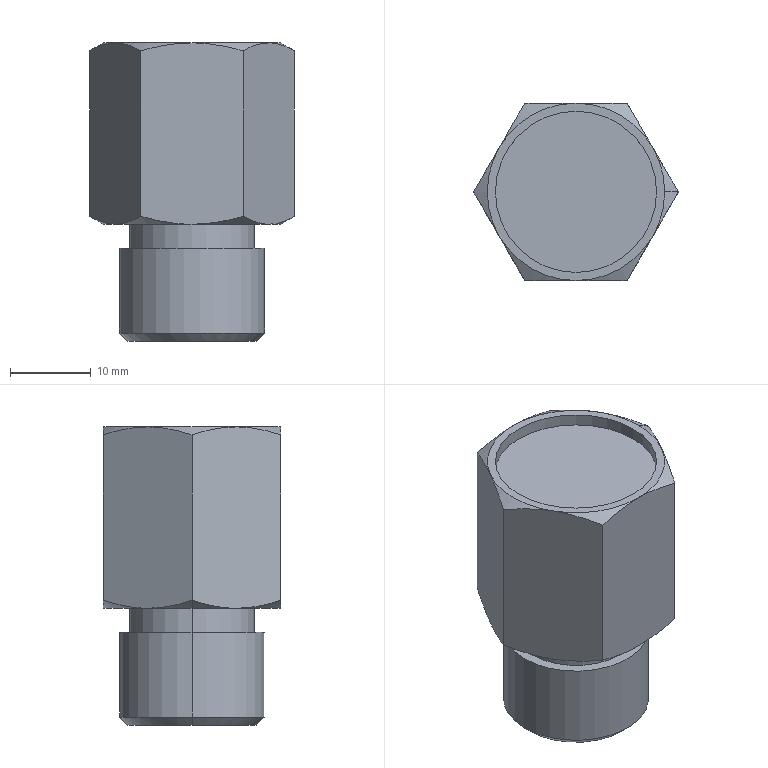Part | SolidWorks | features BaseBody 1 | 1 solid | 36 faces | box 25.403 x 22 x 37 mm | volume 8726 mm3 | cone 16 | plane 12 | cylinder 8 | commonest cylinder face diameters 12 x2 15.5 x2 18 x2 20 x2
STEP:
#1=CARTESIAN_POINT('',(180.5,0.,57.15));
#2=VERTEX_POINT('',#1);
#3=CARTESIAN_POINT('',(164.5,0.,57.15));
#4=VERTEX_POINT('',#3);
#5=CARTESIAN_POINT('',(172.5,0.,57.15));
#6=DIRECTION('',(0.,0.,-1.));
#7=DIRECTION('',(-1.,0.,0.));
#8=AXIS2_PLACEMENT_3D('',#5,#6,#7);
#9=CIRCLE('',#8,8.);
#10=EDGE_CURVE('',#2,#4,#9,.T.);
#11=ORIENTED_EDGE('',*,*,#10,.F.);
#12=CARTESIAN_POINT('',(181.5,0.,58.15));
#13=VERTEX_POINT('',#12);
#14=CARTESIAN_POINT('',(180.5,0.,57.15));
#15=DIRECTION('',(0.7071,0.,0.7071));
#16=VECTOR('',#15,1000.);
#17=LINE('',#14,#16);
#18=EDGE_CURVE('',#2,#13,#17,.T.);
#19=ORIENTED_EDGE('',*,*,#18,.T.);
#20=CARTESIAN_POINT('',(163.5,0.,58.15));
#21=VERTEX_POINT('',#20);
#22=CARTESIAN_POINT('',(172.5,0.,58.15));
#23=DIRECTION('',(0.,0.,1.));
#24=DIRECTION('',(-1.,0.,0.));
#25=AXIS2_PLACEMENT_3D('',#22,#23,#24);
#26=CIRCLE('',#25,9.);
#27=EDGE_CURVE('',#21,#13,#26,.T.);
#28=ORIENTED_EDGE('',*,*,#27,.F.);
#29=CARTESIAN_POINT('',(164.5,0.,57.15));
#30=DIRECTION('',(-0.7071,0.,0.7071));
#31=VECTOR('',#30,1000.);
#32=LINE('',#29,#31);
#33=EDGE_CURVE('',#4,#21,#32,.T.);
#34=ORIENTED_EDGE('',*,*,#33,.F.);
#35=EDGE_LOOP('',(#11,#19,#28,#34));
#36=FACE_OUTER_BOUND('',#35,.T.);
#37=CARTESIAN_POINT('',(172.5,0.,57.15));
#38=DIRECTION('',(0.,0.,1.));
#39=DIRECTION('',(-1.,0.,0.));
#40=AXIS2_PLACEMENT_3D('',#37,#38,#39);
#41=CONICAL_SURFACE('',#40,8.,0.7854);
#42=ADVANCED_FACE('',(#36),#41,.T.);
#43=CARTESIAN_POINT('',(166.5,0.,89.65));
#44=VERTEX_POINT('',#43);
#45=CARTESIAN_POINT('',(178.5,0.,89.65));
#46=VERTEX_POINT('',#45);
#47=CARTESIAN_POINT('',(172.5,0.,89.65));
#48=DIRECTION('',(0.,0.,-1.));
#49=DIRECTION('',(1.,0.,0.));
#50=AXIS2_PLACEMENT_3D('',#47,#48,#49);
#51=CIRCLE('',#50,6.);
#52=EDGE_CURVE('',#44,#46,#51,.T.);
#53=ORIENTED_EDGE('',*,*,#52,.F.);
#54=CARTESIAN_POINT('',(166.5,0.,57.15));
#55=VERTEX_POINT('',#54);
#56=CARTESIAN_POINT('',(166.5,0.,89.65));
#57=DIRECTION('',(0.,0.,-1.));
#58=VECTOR('',#57,1000.);
#59=LINE('',#56,#58);
#60=EDGE_CURVE('',#44,#55,#59,.T.);
#61=ORIENTED_EDGE('',*,*,#60,.T.);
#62=CARTESIAN_POINT('',(178.5,0.,57.15));
#63=VERTEX_POINT('',#62);
#64=CARTESIAN_POINT('',(172.5,0.,57.15));
#65=DIRECTION('',(0.,0.,-1.));
#66=DIRECTION('',(1.,0.,0.));
#67=AXIS2_PLACEMENT_3D('',#64,#65,#66);
#68=CIRCLE('',#67,6.);
#69=EDGE_CURVE('',#55,#63,#68,.T.);
#70=ORIENTED_EDGE('',*,*,#69,.T.);
#71=CARTESIAN_POINT('',(178.5,0.,89.65));
#72=DIRECTION('',(0.,0.,-1.));
#73=VECTOR('',#72,1000.);
#74=LINE('',#71,#73);
#75=EDGE_CURVE('',#46,#63,#74,.T.);
#76=ORIENTED_EDGE('',*,*,#75,.F.);
#77=EDGE_LOOP('',(#53,#61,#70,#76));
#78=FACE_OUTER_BOUND('',#77,.T.);
#79=CARTESIAN_POINT('',(172.5,0.,89.65));
#80=DIRECTION('',(0.,0.,-1.));
#81=DIRECTION('',(1.,0.,0.));
#82=AXIS2_PLACEMENT_3D('',#79,#80,#81);
#83=CYLINDRICAL_SURFACE('',#82,6.);
#84=ADVANCED_FACE('',(#78),#83,.F.);
#85=CARTESIAN_POINT('',(163.5,0.,68.65));
#86=VERTEX_POINT('',#85);
#87=CARTESIAN_POINT('',(181.5,0.,68.65));
#88=VERTEX_POINT('',#87);
#89=CARTESIAN_POINT('',(172.5,0.,68.65));
#90=DIRECTION('',(0.,0.,1.));
#91=DIRECTION('',(-1.,0.,0.));
#92=AXIS2_PLACEMENT_3D('',#89,#90,#91);
#93=CIRCLE('',#92,9.);
#94=EDGE_CURVE('',#86,#88,#93,.T.);
#95=ORIENTED_EDGE('',*,*,#94,.F.);
#96=CARTESIAN_POINT('',(163.5,0.,71.65));
#97=DIRECTION('',(0.,0.,-1.));
#98=VECTOR('',#97,1000.);
#99=LINE('',#96,#98);
#100=EDGE_CURVE('',#86,#21,#99,.T.);
#101=ORIENTED_EDGE('',*,*,#100,.T.);
#102=ORIENTED_EDGE('',*,*,#27,.T.);
#103=CARTESIAN_POINT('',(181.5,0.,71.65));
#104=DIRECTION('',(0.,0.,-1.));
#105=VECTOR('',#104,1000.);
#106=LINE('',#103,#105);
#107=EDGE_CURVE('',#88,#13,#106,.T.);
#108=ORIENTED_EDGE('',*,*,#107,.F.);
#109=EDGE_LOOP('',(#95,#101,#102,#108));
#110=FACE_OUTER_BOUND('',#109,.T.);
#111=CARTESIAN_POINT('',(172.5,0.,71.65));
#112=DIRECTION('',(0.,0.,-1.));
#113=DIRECTION('',(1.,0.,0.));
#114=AXIS2_PLACEMENT_3D('',#111,#112,#113);
#115=CYLINDRICAL_SURFACE('',#114,9.);
#116=ADVANCED_FACE('',(#110),#115,.T.);
#117=CARTESIAN_POINT('',(164.75,0.,68.65));
#118=VERTEX_POINT('',#117);
#119=CARTESIAN_POINT('',(180.25,0.,68.65));
#120=VERTEX_POINT('',#119);
#121=CARTESIAN_POINT('',(172.5,0.,68.65));
#122=DIRECTION('',(0.,0.,1.));
#123=DIRECTION('',(-1.,0.,0.));
#124=AXIS2_PLACEMENT_3D('',#121,#122,#123);
#125=CIRCLE('',#124,7.75);
#126=EDGE_CURVE('',#118,#120,#125,.T.);
#127=ORIENTED_EDGE('',*,*,#126,.T.);
#128=CARTESIAN_POINT('',(180.25,0.,71.65));
#129=VERTEX_POINT('',#128);
#130=CARTESIAN_POINT('',(180.25,0.,94.15));
#131=DIRECTION('',(0.,0.,1.));
#132=VECTOR('',#131,1000.);
#133=LINE('',#130,#132);
#134=EDGE_CURVE('',#120,#129,#133,.T.);
#135=ORIENTED_EDGE('',*,*,#134,.T.);
#136=CARTESIAN_POINT('',(164.75,0.,71.65));
#137=VERTEX_POINT('',#136);
#138=CARTESIAN_POINT('',(172.5,0.,71.65));
#139=DIRECTION('',(0.,0.,1.));
#140=DIRECTION('',(-1.,0.,0.));
#141=AXIS2_PLACEMENT_3D('',#138,#139,#140);
#142=CIRCLE('',#141,7.75);
#143=EDGE_CURVE('',#137,#129,#142,.T.);
#144=ORIENTED_EDGE('',*,*,#143,.F.);
#145=CARTESIAN_POINT('',(164.75,0.,94.15));
#146=DIRECTION('',(0.,0.,1.));
#147=VECTOR('',#146,1000.);
#148=LINE('',#145,#147);
#149=EDGE_CURVE('',#118,#137,#148,.T.);
#150=ORIENTED_EDGE('',*,*,#149,.F.);
#151=EDGE_LOOP('',(#127,#135,#144,#150));
#152=FACE_OUTER_BOUND('',#151,.T.);
#153=CARTESIAN_POINT('',(172.5,0.,94.15));
#154=DIRECTION('',(0.,0.,1.));
#155=DIRECTION('',(-1.,0.,0.));
#156=AXIS2_PLACEMENT_3D('',#153,#154,#155);
#157=CYLINDRICAL_SURFACE('',#156,7.75);
#158=ADVANCED_FACE('',(#152),#157,.T.);
#159=CARTESIAN_POINT('',(182.5,0.,92.65));
#160=VERTEX_POINT('',#159);
#161=CARTESIAN_POINT('',(162.5,0.,92.65));
#162=VERTEX_POINT('',#161);
#163=CARTESIAN_POINT('',(172.5,0.,92.65));
#164=DIRECTION('',(0.,0.,1.));
#165=DIRECTION('',(-1.,0.,0.));
#166=AXIS2_PLACEMENT_3D('',#163,#164,#165);
#167=CIRCLE('',#166,10.);
#168=EDGE_CURVE('',#160,#162,#167,.T.);
#169=ORIENTED_EDGE('',*,*,#168,.F.);
#170=CARTESIAN_POINT('',(182.5,0.,94.15));
#171=VERTEX_POINT('',#170);
#172=CARTESIAN_POINT('',(182.5,0.,92.65));
#173=DIRECTION('',(0.,0.,1.));
#174=VECTOR('',#173,1000.);
#175=LINE('',#172,#174);
#176=EDGE_CURVE('',#160,#171,#175,.T.);
#177=ORIENTED_EDGE('',*,*,#176,.T.);
#178=CARTESIAN_POINT('',(162.5,0.,94.15));
#179=VERTEX_POINT('',#178);
#180=CARTESIAN_POINT('',(172.5,0.,94.15));
#181=DIRECTION('',(0.,0.,1.));
#182=DIRECTION('',(-1.,0.,0.));
#183=AXIS2_PLACEMENT_3D('',#180,#181,#182);
#184=CIRCLE('',#183,10.);
#185=EDGE_CURVE('',#171,#179,#184,.T.);
#186=ORIENTED_EDGE('',*,*,#185,.T.);
#187=CARTESIAN_POINT('',(162.5,0.,92.65));
#188=DIRECTION('',(0.,0.,1.));
#189=VECTOR('',#188,1000.);
#190=LINE('',#187,#189);
#191=EDGE_CURVE('',#162,#179,#190,.T.);
#192=ORIENTED_EDGE('',*,*,#191,.F.);
#193=EDGE_LOOP('',(#169,#177,#186,#192));
#194=FACE_OUTER_BOUND('',#193,.T.);
#195=CARTESIAN_POINT('',(172.5,0.,92.65));
#196=DIRECTION('',(0.,0.,1.));
#197=DIRECTION('',(-1.,0.,0.));
#198=AXIS2_PLACEMENT_3D('',#195,#196,#197);
#199=CYLINDRICAL_SURFACE('',#198,10.);
#200=ADVANCED_FACE('',(#194),#199,.F.);
#201=CARTESIAN_POINT('',(183.5,0.,94.15));
#202=VERTEX_POINT('',#201);
#203=CARTESIAN_POINT('',(182.026,5.5,94.15));
#204=VERTEX_POINT('',#203);
#205=CARTESIAN_POINT('',(172.5,0.,94.15));
#206=DIRECTION('',(0.,0.,1.));
#207=DIRECTION('',(-1.,0.,0.));
#208=AXIS2_PLACEMENT_3D('',#205,#206,#207);
#209=CIRCLE('',#208,11.);
#210=EDGE_CURVE('',#202,#204,#209,.T.);
#211=ORIENTED_EDGE('',*,*,#210,.F.);
#212=CARTESIAN_POINT('',(185.202,0.,93.168));
#213=VERTEX_POINT('',#212);
#214=CARTESIAN_POINT('',(183.5,0.,94.15));
#215=DIRECTION('',(0.866,0.,-0.5));
#216=VECTOR('',#215,1000.);
#217=LINE('',#214,#216);
#218=EDGE_CURVE('',#202,#213,#217,.T.);
#219=ORIENTED_EDGE('',*,*,#218,.T.);
#220=CARTESIAN_POINT('',(185.202,0.,93.168));
#221=CARTESIAN_POINT('',(184.682,0.8997,93.467));
#222=CARTESIAN_POINT('',(184.159,1.806,93.715));
#223=CARTESIAN_POINT('',(183.102,3.638,94.056));
#224=CARTESIAN_POINT('',(182.567,4.563,94.15));
#225=CARTESIAN_POINT('',(182.026,5.5,94.15));
#226=B_SPLINE_CURVE_WITH_KNOTS('',3,(#220,#221,#222,#223,#224,#225),.UNSPECIFIED.,.F.,.F.,(4,2,4),(0.000000238,0.003213,0.006426),.UNSPECIFIED.);
#227=EDGE_CURVE('',#213,#204,#226,.T.);
#228=ORIENTED_EDGE('',*,*,#227,.T.);
#229=EDGE_LOOP('',(#211,#219,#228));
#230=FACE_OUTER_BOUND('',#229,.T.);
#231=CARTESIAN_POINT('',(172.5,0.,94.15));
#232=DIRECTION('',(0.,0.,-1.));
#233=DIRECTION('',(1.,0.,0.));
#234=AXIS2_PLACEMENT_3D('',#231,#232,#233);
#235=CONICAL_SURFACE('',#234,11.,1.047);
#236=ADVANCED_FACE('',(#230),#235,.T.);
#237=CARTESIAN_POINT('',(161.5,0.,71.65));
#238=VERTEX_POINT('',#237);
#239=CARTESIAN_POINT('',(162.974,5.5,71.65));
#240=VERTEX_POINT('',#239);
#241=CARTESIAN_POINT('',(172.5,0.,71.65));
#242=DIRECTION('',(0.,0.,-1.));
#243=DIRECTION('',(1.,0.,0.));
#244=AXIS2_PLACEMENT_3D('',#241,#242,#243);
#245=CIRCLE('',#244,11.);
#246=EDGE_CURVE('',#238,#240,#245,.T.);
#247=ORIENTED_EDGE('',*,*,#246,.F.);
#248=CARTESIAN_POINT('',(159.798,0.,72.632));
#249=VERTEX_POINT('',#248);
#250=CARTESIAN_POINT('',(159.798,0.,72.632));
#251=DIRECTION('',(-0.866,0.,0.5));
#252=VECTOR('',#251,1000.);
#253=LINE('',#250,#252);
#254=EDGE_CURVE('',#238,#249,#253,.T.);
#255=ORIENTED_EDGE('',*,*,#254,.T.);
#256=CARTESIAN_POINT('',(159.798,0.,72.632));
#257=CARTESIAN_POINT('',(160.318,0.8997,72.333));
#258=CARTESIAN_POINT('',(160.841,1.806,72.085));
#259=CARTESIAN_POINT('',(161.898,3.638,71.744));
#260=CARTESIAN_POINT('',(162.433,4.563,71.65));
#261=CARTESIAN_POINT('',(162.974,5.5,71.65));
#262=B_SPLINE_CURVE_WITH_KNOTS('',3,(#256,#257,#258,#259,#260,#261),.UNSPECIFIED.,.F.,.F.,(4,2,4),(0.000000238,0.003213,0.006426),.UNSPECIFIED.);
#263=EDGE_CURVE('',#249,#240,#262,.T.);
#264=ORIENTED_EDGE('',*,*,#263,.T.);
#265=EDGE_LOOP('',(#247,#255,#264));
#266=FACE_OUTER_BOUND('',#265,.T.);
#267=CARTESIAN_POINT('',(172.5,0.,72.632));
#268=DIRECTION('',(0.,0.,1.));
#269=DIRECTION('',(-1.,0.,0.));
#270=AXIS2_PLACEMENT_3D('',#267,#268,#269);
#271=CONICAL_SURFACE('',#270,12.702,1.047);
#272=ADVANCED_FACE('',(#266),#271,.T.);
#273=CARTESIAN_POINT('',(159.798,0.,93.168));
#274=VERTEX_POINT('',#273);
#275=CARTESIAN_POINT('',(162.974,-5.5,94.15));
#276=VERTEX_POINT('',#275);
#277=CARTESIAN_POINT('',(159.798,0.,93.168));
#278=CARTESIAN_POINT('',(160.318,-0.8997,93.467));
#279=CARTESIAN_POINT('',(160.841,-1.806,93.715));
#280=CARTESIAN_POINT('',(161.898,-3.638,94.056));
#281=CARTESIAN_POINT('',(162.433,-4.563,94.15));
#282=CARTESIAN_POINT('',(162.974,-5.5,94.15));
#283=B_SPLINE_CURVE_WITH_KNOTS('',3,(#277,#278,#279,#280,#281,#282),.UNSPECIFIED.,.F.,.F.,(4,2,4),(0.000000238,0.003213,0.006426),.UNSPECIFIED.);
#284=EDGE_CURVE('',#274,#276,#283,.T.);
#285=ORIENTED_EDGE('',*,*,#284,.F.);
#286=CARTESIAN_POINT('',(159.798,0.,57.15));
#287=DIRECTION('',(0.,0.,1.));
#288=VECTOR('',#287,1000.);
#289=LINE('',#286,#288);
#290=EDGE_CURVE('',#249,#274,#289,.T.);
#291=ORIENTED_EDGE('',*,*,#290,.F.);
#292=CARTESIAN_POINT('',(162.974,-5.5,71.65));
#293=VERTEX_POINT('',#292);
#294=CARTESIAN_POINT('',(162.974,-5.5,71.65));
#295=CARTESIAN_POINT('',(162.704,-5.033,71.65));
#296=CARTESIAN_POINT('',(162.434,-4.564,71.673));
#297=CARTESIAN_POINT('',(161.898,-3.637,71.763));
#298=CARTESIAN_POINT('',(161.632,-3.176,71.83));
#299=CARTESIAN_POINT('',(160.839,-1.802,72.086));
#300=CARTESIAN_POINT('',(160.316,-0.8975,72.333));
#301=CARTESIAN_POINT('',(159.798,0.,72.632));
#302=B_SPLINE_CURVE_WITH_KNOTS('',3,(#294,#295,#296,#297,#298,#299,#300,#301),.UNSPECIFIED.,.F.,.F.,(4,2,2,4),(0.006426,0.008027,0.009627,0.01283),.UNSPECIFIED.);
#303=EDGE_CURVE('',#293,#249,#302,.T.);
#304=ORIENTED_EDGE('',*,*,#303,.F.);
#305=CARTESIAN_POINT('',(166.149,-11.,72.632));
#306=VERTEX_POINT('',#305);
#307=CARTESIAN_POINT('',(166.149,-11.,72.632));
#308=CARTESIAN_POINT('',(165.63,-10.1,72.333));
#309=CARTESIAN_POINT('',(165.106,-9.194,72.085));
#310=CARTESIAN_POINT('',(164.049,-7.362,71.744));
#311=CARTESIAN_POINT('',(163.515,-6.437,71.65));
#312=CARTESIAN_POINT('',(162.974,-5.5,71.65));
#313=B_SPLINE_CURVE_WITH_KNOTS('',3,(#307,#308,#309,#310,#311,#312),.UNSPECIFIED.,.F.,.F.,(4,2,4),(0.000000238,0.003213,0.006426),.UNSPECIFIED.);
#314=EDGE_CURVE('',#306,#293,#313,.T.);
#315=ORIENTED_EDGE('',*,*,#314,.F.);
#316=CARTESIAN_POINT('',(166.149,-11.,93.168));
#317=VERTEX_POINT('',#316);
#318=CARTESIAN_POINT('',(166.149,-11.,57.15));
#319=DIRECTION('',(0.,0.,1.));
#320=VECTOR('',#319,1000.);
#321=LINE('',#318,#320);
#322=EDGE_CURVE('',#306,#317,#321,.T.);
#323=ORIENTED_EDGE('',*,*,#322,.T.);
#324=CARTESIAN_POINT('',(162.974,-5.5,94.15));
#325=CARTESIAN_POINT('',(163.243,-5.967,94.15));
#326=CARTESIAN_POINT('',(163.514,-6.436,94.127));
#327=CARTESIAN_POINT('',(164.049,-7.363,94.037));
#328=CARTESIAN_POINT('',(164.315,-7.824,93.97));
#329=CARTESIAN_POINT('',(165.109,-9.198,93.714));
#330=CARTESIAN_POINT('',(165.631,-10.103,93.467));
#331=CARTESIAN_POINT('',(166.149,-11.,93.168));
#332=B_SPLINE_CURVE_WITH_KNOTS('',3,(#324,#325,#326,#327,#328,#329,#330,#331),.UNSPECIFIED.,.F.,.F.,(4,2,2,4),(0.006426,0.008027,0.009627,0.01283),.UNSPECIFIED.);
#333=EDGE_CURVE('',#276,#317,#332,.T.);
#334=ORIENTED_EDGE('',*,*,#333,.F.);
#335=EDGE_LOOP('',(#285,#291,#304,#315,#323,#334));
#336=FACE_OUTER_BOUND('',#335,.T.);
#337=CARTESIAN_POINT('',(166.149,-11.,57.15));
#338=DIRECTION('',(0.866,0.5,0.));
#339=DIRECTION('',(0.5,-0.866,0.));
#340=AXIS2_PLACEMENT_3D('',#337,#338,#339);
#341=PLANE('',#340);
#342=ADVANCED_FACE('',(#336),#341,.F.);
#343=CARTESIAN_POINT('',(166.149,11.,93.168));
#344=VERTEX_POINT('',#343);
#345=CARTESIAN_POINT('',(162.974,5.5,94.15));
#346=VERTEX_POINT('',#345);
#347=CARTESIAN_POINT('',(166.149,11.,93.168));
#348=CARTESIAN_POINT('',(165.63,10.1,93.467));
#349=CARTESIAN_POINT('',(165.106,9.194,93.715));
#350=CARTESIAN_POINT('',(164.049,7.362,94.056));
#351=CARTESIAN_POINT('',(163.515,6.437,94.15));
#352=CARTESIAN_POINT('',(162.974,5.5,94.15));
#353=B_SPLINE_CURVE_WITH_KNOTS('',3,(#347,#348,#349,#350,#351,#352),.UNSPECIFIED.,.F.,.F.,(4,2,4),(0.000000238,0.003213,0.006426),.UNSPECIFIED.);
#354=EDGE_CURVE('',#344,#346,#353,.T.);
#355=ORIENTED_EDGE('',*,*,#354,.F.);
#356=CARTESIAN_POINT('',(166.149,11.,72.632));
#357=VERTEX_POINT('',#356);
#358=CARTESIAN_POINT('',(166.149,11.,57.15));
#359=DIRECTION('',(0.,0.,1.));
#360=VECTOR('',#359,1000.);
#361=LINE('',#358,#360);
#362=EDGE_CURVE('',#357,#344,#361,.T.);
#363=ORIENTED_EDGE('',*,*,#362,.F.);
#364=CARTESIAN_POINT('',(162.974,5.5,71.65));
#365=CARTESIAN_POINT('',(163.243,5.967,71.65));
#366=CARTESIAN_POINT('',(163.514,6.436,71.673));
#367=CARTESIAN_POINT('',(164.049,7.363,71.763));
#368=CARTESIAN_POINT('',(164.315,7.824,71.83));
#369=CARTESIAN_POINT('',(165.109,9.198,72.086));
#370=CARTESIAN_POINT('',(165.631,10.103,72.333));
#371=CARTESIAN_POINT('',(166.149,11.,72.632));
#372=B_SPLINE_CURVE_WITH_KNOTS('',3,(#364,#365,#366,#367,#368,#369,#370,#371),.UNSPECIFIED.,.F.,.F.,(4,2,2,4),(0.006426,0.008027,0.009627,0.01283),.UNSPECIFIED.);
#373=EDGE_CURVE('',#240,#357,#372,.T.);
#374=ORIENTED_EDGE('',*,*,#373,.F.);
#375=ORIENTED_EDGE('',*,*,#263,.F.);
#376=ORIENTED_EDGE('',*,*,#290,.T.);
#377=CARTESIAN_POINT('',(162.974,5.5,94.15));
#378=CARTESIAN_POINT('',(162.704,5.033,94.15));
#379=CARTESIAN_POINT('',(162.434,4.564,94.127));
#380=CARTESIAN_POINT('',(161.898,3.637,94.037));
#381=CARTESIAN_POINT('',(161.632,3.176,93.97));
#382=CARTESIAN_POINT('',(160.839,1.802,93.714));
#383=CARTESIAN_POINT('',(160.316,0.8975,93.467));
#384=CARTESIAN_POINT('',(159.798,0.,93.168));
#385=B_SPLINE_CURVE_WITH_KNOTS('',3,(#377,#378,#379,#380,#381,#382,#383,#384),.UNSPECIFIED.,.F.,.F.,(4,2,2,4),(0.006426,0.008027,0.009627,0.01283),.UNSPECIFIED.);
#386=EDGE_CURVE('',#346,#274,#385,.T.);
#387=ORIENTED_EDGE('',*,*,#386,.F.);
#388=EDGE_LOOP('',(#355,#363,#374,#375,#376,#387));
#389=FACE_OUTER_BOUND('',#388,.T.);
#390=CARTESIAN_POINT('',(159.798,0.,57.15));
#391=DIRECTION('',(0.866,-0.5,0.));
#392=DIRECTION('',(-0.5,-0.866,0.));
#393=AXIS2_PLACEMENT_3D('',#390,#391,#392);
#394=PLANE('',#393);
#395=ADVANCED_FACE('',(#389),#394,.F.);
#396=CARTESIAN_POINT('',(178.851,11.,93.168));
#397=VERTEX_POINT('',#396);
#398=CARTESIAN_POINT('',(172.5,11.,94.15));
#399=VERTEX_POINT('',#398);
#400=CARTESIAN_POINT('',(178.851,11.,93.168));
#401=CARTESIAN_POINT('',(177.824,11.,93.464));
#402=CARTESIAN_POINT('',(176.784,11.,93.711));
#403=CARTESIAN_POINT('',(175.193,11.,93.969));
#404=CARTESIAN_POINT('',(174.656,11.,94.037));
#405=CARTESIAN_POINT('',(173.576,11.,94.127));
#406=CARTESIAN_POINT('',(173.037,11.,94.15));
#407=CARTESIAN_POINT('',(172.5,11.,94.15));
#408=B_SPLINE_CURVE_WITH_KNOTS('',3,(#400,#401,#402,#403,#404,#405,#406,#407),.UNSPECIFIED.,.F.,.F.,(4,2,2,4),(0.004655,0.007861,0.009464,0.01107),.UNSPECIFIED.);
#409=EDGE_CURVE('',#397,#399,#408,.T.);
#410=ORIENTED_EDGE('',*,*,#409,.F.);
#411=CARTESIAN_POINT('',(178.851,11.,72.632));
#412=VERTEX_POINT('',#411);
#413=CARTESIAN_POINT('',(178.851,11.,57.15));
#414=DIRECTION('',(0.,0.,1.));
#415=VECTOR('',#414,1000.);
#416=LINE('',#413,#415);
#417=EDGE_CURVE('',#412,#397,#416,.T.);
#418=ORIENTED_EDGE('',*,*,#417,.F.);
#419=CARTESIAN_POINT('',(172.5,11.,71.65));
#420=VERTEX_POINT('',#419);
#421=CARTESIAN_POINT('',(172.5,11.,71.65));
#422=CARTESIAN_POINT('',(173.037,11.,71.65));
#423=CARTESIAN_POINT('',(173.576,11.,71.673));
#424=CARTESIAN_POINT('',(174.656,11.,71.763));
#425=CARTESIAN_POINT('',(175.193,11.,71.831));
#426=CARTESIAN_POINT('',(176.784,11.,72.089));
#427=CARTESIAN_POINT('',(177.824,11.,72.336));
#428=CARTESIAN_POINT('',(178.851,11.,72.632));
#429=B_SPLINE_CURVE_WITH_KNOTS('',3,(#421,#422,#423,#424,#425,#426,#427,#428),.UNSPECIFIED.,.F.,.F.,(4,2,2,4),(0.01776,0.01936,0.02097,0.02418),.UNSPECIFIED.);
#430=EDGE_CURVE('',#420,#412,#429,.T.);
#431=ORIENTED_EDGE('',*,*,#430,.F.);
#432=CARTESIAN_POINT('',(166.149,11.,72.632));
#433=CARTESIAN_POINT('',(167.182,11.,72.334));
#434=CARTESIAN_POINT('',(168.24,11.,72.084));
#435=CARTESIAN_POINT('',(170.361,11.,71.742));
#436=CARTESIAN_POINT('',(171.427,11.,71.65));
#437=CARTESIAN_POINT('',(172.5,11.,71.65));
#438=B_SPLINE_CURVE_WITH_KNOTS('',3,(#432,#433,#434,#435,#436,#437),.UNSPECIFIED.,.F.,.F.,(4,2,4),(0.01133,0.01454,0.01776),.UNSPECIFIED.);
#439=EDGE_CURVE('',#357,#420,#438,.T.);
#440=ORIENTED_EDGE('',*,*,#439,.F.);
#441=ORIENTED_EDGE('',*,*,#362,.T.);
#442=CARTESIAN_POINT('',(172.5,11.,94.15));
#443=CARTESIAN_POINT('',(171.427,11.,94.15));
#444=CARTESIAN_POINT('',(170.361,11.,94.058));
#445=CARTESIAN_POINT('',(168.24,11.,93.716));
#446=CARTESIAN_POINT('',(167.182,11.,93.466));
#447=CARTESIAN_POINT('',(166.149,11.,93.168));
#448=B_SPLINE_CURVE_WITH_KNOTS('',3,(#442,#443,#444,#445,#446,#447),.UNSPECIFIED.,.F.,.F.,(4,2,4),(0.01107,0.01427,0.01748),.UNSPECIFIED.);
#449=EDGE_CURVE('',#399,#344,#448,.T.);
#450=ORIENTED_EDGE('',*,*,#449,.F.);
#451=EDGE_LOOP('',(#410,#418,#431,#440,#441,#450));
#452=FACE_OUTER_BOUND('',#451,.T.);
#453=CARTESIAN_POINT('',(166.149,11.,57.15));
#454=DIRECTION('',(0.,-1.,0.));
#455=DIRECTION('',(-1.,0.,0.));
#456=AXIS2_PLACEMENT_3D('',#453,#454,#455);
#457=PLANE('',#456);
#458=ADVANCED_FACE('',(#452),#457,.F.);
#459=ORIENTED_EDGE('',*,*,#227,.F.);
#460=CARTESIAN_POINT('',(185.202,0.,72.632));
#461=VERTEX_POINT('',#460);
#462=CARTESIAN_POINT('',(185.202,0.,57.15));
#463=DIRECTION('',(0.,0.,1.));
#464=VECTOR('',#463,1000.);
#465=LINE('',#462,#464);
#466=EDGE_CURVE('',#461,#213,#465,.T.);
#467=ORIENTED_EDGE('',*,*,#466,.F.);
#468=CARTESIAN_POINT('',(182.026,5.5,71.65));
#469=VERTEX_POINT('',#468);
#470=CARTESIAN_POINT('',(182.026,5.5,71.65));
#471=CARTESIAN_POINT('',(182.296,5.033,71.65));
#472=CARTESIAN_POINT('',(182.566,4.564,71.673));
#473=CARTESIAN_POINT('',(183.102,3.637,71.763));
#474=CARTESIAN_POINT('',(183.368,3.176,71.83));
#475=CARTESIAN_POINT('',(184.161,1.802,72.086));
#476=CARTESIAN_POINT('',(184.684,0.8975,72.333));
#477=CARTESIAN_POINT('',(185.202,0.,72.632));
#478=B_SPLINE_CURVE_WITH_KNOTS('',3,(#470,#471,#472,#473,#474,#475,#476,#477),.UNSPECIFIED.,.F.,.F.,(4,2,2,4),(0.006426,0.008027,0.009627,0.01283),.UNSPECIFIED.);
#479=EDGE_CURVE('',#469,#461,#478,.T.);
#480=ORIENTED_EDGE('',*,*,#479,.F.);
#481=CARTESIAN_POINT('',(178.851,11.,72.632));
#482=CARTESIAN_POINT('',(179.37,10.1,72.333));
#483=CARTESIAN_POINT('',(179.894,9.194,72.085));
#484=CARTESIAN_POINT('',(180.951,7.362,71.744));
#485=CARTESIAN_POINT('',(181.485,6.437,71.65));
#486=CARTESIAN_POINT('',(182.026,5.5,71.65));
#487=B_SPLINE_CURVE_WITH_KNOTS('',3,(#481,#482,#483,#484,#485,#486),.UNSPECIFIED.,.F.,.F.,(4,2,4),(0.000000238,0.003213,0.006426),.UNSPECIFIED.);
#488=EDGE_CURVE('',#412,#469,#487,.T.);
#489=ORIENTED_EDGE('',*,*,#488,.F.);
#490=ORIENTED_EDGE('',*,*,#417,.T.);
#491=CARTESIAN_POINT('',(182.026,5.5,94.15));
#492=CARTESIAN_POINT('',(181.757,5.967,94.15));
#493=CARTESIAN_POINT('',(181.486,6.436,94.127));
#494=CARTESIAN_POINT('',(180.951,7.363,94.037));
#495=CARTESIAN_POINT('',(180.685,7.824,93.97));
#496=CARTESIAN_POINT('',(179.891,9.198,93.714));
#497=CARTESIAN_POINT('',(179.369,10.103,93.467));
#498=CARTESIAN_POINT('',(178.851,11.,93.168));
#499=B_SPLINE_CURVE_WITH_KNOTS('',3,(#491,#492,#493,#494,#495,#496,#497,#498),.UNSPECIFIED.,.F.,.F.,(4,2,2,4),(0.006426,0.008027,0.009627,0.01283),.UNSPECIFIED.);
#500=EDGE_CURVE('',#204,#397,#499,.T.);
#501=ORIENTED_EDGE('',*,*,#500,.F.);
#502=EDGE_LOOP('',(#459,#467,#480,#489,#490,#501));
#503=FACE_OUTER_BOUND('',#502,.T.);
#504=CARTESIAN_POINT('',(178.851,11.,57.15));
#505=DIRECTION('',(-0.866,-0.5,0.));
#506=DIRECTION('',(-0.5,0.866,0.));
#507=AXIS2_PLACEMENT_3D('',#504,#505,#506);
#508=PLANE('',#507);
#509=ADVANCED_FACE('',(#503),#508,.F.);
#510=CARTESIAN_POINT('',(178.851,-11.,93.168));
#511=VERTEX_POINT('',#510);
#512=CARTESIAN_POINT('',(182.026,-5.5,94.15));
#513=VERTEX_POINT('',#512);
#514=CARTESIAN_POINT('',(178.851,-11.,93.168));
#515=CARTESIAN_POINT('',(179.37,-10.1,93.467));
#516=CARTESIAN_POINT('',(179.894,-9.194,93.715));
#517=CARTESIAN_POINT('',(180.951,-7.362,94.056));
#518=CARTESIAN_POINT('',(181.485,-6.437,94.15));
#519=CARTESIAN_POINT('',(182.026,-5.5,94.15));
#520=B_SPLINE_CURVE_WITH_KNOTS('',3,(#514,#515,#516,#517,#518,#519),.UNSPECIFIED.,.F.,.F.,(4,2,4),(0.000000238,0.003213,0.006426),.UNSPECIFIED.);
#521=EDGE_CURVE('',#511,#513,#520,.T.);
#522=ORIENTED_EDGE('',*,*,#521,.F.);
#523=CARTESIAN_POINT('',(178.851,-11.,72.632));
#524=VERTEX_POINT('',#523);
#525=CARTESIAN_POINT('',(178.851,-11.,57.15));
#526=DIRECTION('',(0.,0.,1.));
#527=VECTOR('',#526,1000.);
#528=LINE('',#525,#527);
#529=EDGE_CURVE('',#524,#511,#528,.T.);
#530=ORIENTED_EDGE('',*,*,#529,.F.);
#531=CARTESIAN_POINT('',(182.026,-5.5,71.65));
#532=VERTEX_POINT('',#531);
#533=CARTESIAN_POINT('',(182.026,-5.5,71.65));
#534=CARTESIAN_POINT('',(181.757,-5.967,71.65));
#535=CARTESIAN_POINT('',(181.486,-6.436,71.673));
#536=CARTESIAN_POINT('',(180.951,-7.363,71.763));
#537=CARTESIAN_POINT('',(180.685,-7.824,71.83));
#538=CARTESIAN_POINT('',(179.891,-9.198,72.086));
#539=CARTESIAN_POINT('',(179.369,-10.103,72.333));
#540=CARTESIAN_POINT('',(178.851,-11.,72.632));
#541=B_SPLINE_CURVE_WITH_KNOTS('',3,(#533,#534,#535,#536,#537,#538,#539,#540),.UNSPECIFIED.,.F.,.F.,(4,2,2,4),(0.006426,0.008027,0.009627,0.01283),.UNSPECIFIED.);
#542=EDGE_CURVE('',#532,#524,#541,.T.);
#543=ORIENTED_EDGE('',*,*,#542,.F.);
#544=CARTESIAN_POINT('',(185.202,0.,72.632));
#545=CARTESIAN_POINT('',(184.682,-0.8997,72.333));
#546=CARTESIAN_POINT('',(184.159,-1.806,72.085));
#547=CARTESIAN_POINT('',(183.102,-3.638,71.744));
#548=CARTESIAN_POINT('',(182.567,-4.563,71.65));
#549=CARTESIAN_POINT('',(182.026,-5.5,71.65));
#550=B_SPLINE_CURVE_WITH_KNOTS('',3,(#544,#545,#546,#547,#548,#549),.UNSPECIFIED.,.F.,.F.,(4,2,4),(0.000000238,0.003213,0.006426),.UNSPECIFIED.);
#551=EDGE_CURVE('',#461,#532,#550,.T.);
#552=ORIENTED_EDGE('',*,*,#551,.F.);
#553=ORIENTED_EDGE('',*,*,#466,.T.);
#554=CARTESIAN_POINT('',(182.026,-5.5,94.15));
#555=CARTESIAN_POINT('',(182.296,-5.033,94.15));
#556=CARTESIAN_POINT('',(182.566,-4.564,94.127));
#557=CARTESIAN_POINT('',(183.102,-3.637,94.037));
#558=CARTESIAN_POINT('',(183.368,-3.176,93.97));
#559=CARTESIAN_POINT('',(184.161,-1.802,93.714));
#560=CARTESIAN_POINT('',(184.684,-0.8975,93.467));
#561=CARTESIAN_POINT('',(185.202,0.,93.168));
#562=B_SPLINE_CURVE_WITH_KNOTS('',3,(#554,#555,#556,#557,#558,#559,#560,#561),.UNSPECIFIED.,.F.,.F.,(4,2,2,4),(0.006426,0.008027,0.009627,0.01283),.UNSPECIFIED.);
#563=EDGE_CURVE('',#513,#213,#562,.T.);
#564=ORIENTED_EDGE('',*,*,#563,.F.);
#565=EDGE_LOOP('',(#522,#530,#543,#552,#553,#564));
#566=FACE_OUTER_BOUND('',#565,.T.);
#567=CARTESIAN_POINT('',(185.202,0.,57.15));
#568=DIRECTION('',(-0.866,0.5,0.));
#569=DIRECTION('',(0.5,0.866,0.));
#570=AXIS2_PLACEMENT_3D('',#567,#568,#569);
#571=PLANE('',#570);
#572=ADVANCED_FACE('',(#566),#571,.F.);
#573=CARTESIAN_POINT('',(172.5,-11.,94.15));
#574=VERTEX_POINT('',#573);
#575=CARTESIAN_POINT('',(166.149,-11.,93.168));
#576=CARTESIAN_POINT('',(167.182,-11.,93.466));
#577=CARTESIAN_POINT('',(168.24,-11.,93.716));
#578=CARTESIAN_POINT('',(170.361,-11.,94.058));
#579=CARTESIAN_POINT('',(171.427,-11.,94.15));
#580=CARTESIAN_POINT('',(172.5,-11.,94.15));
#581=B_SPLINE_CURVE_WITH_KNOTS('',3,(#575,#576,#577,#578,#579,#580),.UNSPECIFIED.,.F.,.F.,(4,2,4),(0.01133,0.01454,0.01776),.UNSPECIFIED.);
#582=EDGE_CURVE('',#317,#574,#581,.T.);
#583=ORIENTED_EDGE('',*,*,#582,.F.);
#584=ORIENTED_EDGE('',*,*,#322,.F.);
#585=CARTESIAN_POINT('',(172.5,-11.,71.65));
#586=VERTEX_POINT('',#585);
#587=CARTESIAN_POINT('',(172.5,-11.,71.65));
#588=CARTESIAN_POINT('',(171.427,-11.,71.65));
#589=CARTESIAN_POINT('',(170.361,-11.,71.742));
#590=CARTESIAN_POINT('',(168.24,-11.,72.084));
#591=CARTESIAN_POINT('',(167.182,-11.,72.334));
#592=CARTESIAN_POINT('',(166.149,-11.,72.632));
#593=B_SPLINE_CURVE_WITH_KNOTS('',3,(#587,#588,#589,#590,#591,#592),.UNSPECIFIED.,.F.,.F.,(4,2,4),(0.01107,0.01427,0.01748),.UNSPECIFIED.);
#594=EDGE_CURVE('',#586,#306,#593,.T.);
#595=ORIENTED_EDGE('',*,*,#594,.F.);
#596=CARTESIAN_POINT('',(178.851,-11.,72.632));
#597=CARTESIAN_POINT('',(177.824,-11.,72.336));
#598=CARTESIAN_POINT('',(176.784,-11.,72.089));
#599=CARTESIAN_POINT('',(175.193,-11.,71.831));
#600=CARTESIAN_POINT('',(174.656,-11.,71.763));
#601=CARTESIAN_POINT('',(173.576,-11.,71.673));
#602=CARTESIAN_POINT('',(173.037,-11.,71.65));
#603=CARTESIAN_POINT('',(172.5,-11.,71.65));
#604=B_SPLINE_CURVE_WITH_KNOTS('',3,(#596,#597,#598,#599,#600,#601,#602,#603),.UNSPECIFIED.,.F.,.F.,(4,2,2,4),(0.004655,0.007861,0.009464,0.01107),.UNSPECIFIED.);
#605=EDGE_CURVE('',#524,#586,#604,.T.);
#606=ORIENTED_EDGE('',*,*,#605,.F.);
#607=ORIENTED_EDGE('',*,*,#529,.T.);
#608=CARTESIAN_POINT('',(172.5,-11.,94.15));
#609=CARTESIAN_POINT('',(173.037,-11.,94.15));
#610=CARTESIAN_POINT('',(173.576,-11.,94.127));
#611=CARTESIAN_POINT('',(174.656,-11.,94.037));
#612=CARTESIAN_POINT('',(175.193,-11.,93.969));
#613=CARTESIAN_POINT('',(176.784,-11.,93.711));
#614=CARTESIAN_POINT('',(177.824,-11.,93.464));
#615=CARTESIAN_POINT('',(178.851,-11.,93.168));
#616=B_SPLINE_CURVE_WITH_KNOTS('',3,(#608,#609,#610,#611,#612,#613,#614,#615),.UNSPECIFIED.,.F.,.F.,(4,2,2,4),(0.01776,0.01936,0.02097,0.02418),.UNSPECIFIED.);
#617=EDGE_CURVE('',#574,#511,#616,.T.);
#618=ORIENTED_EDGE('',*,*,#617,.F.);
#619=EDGE_LOOP('',(#583,#584,#595,#606,#607,#618));
#620=FACE_OUTER_BOUND('',#619,.T.);
#621=CARTESIAN_POINT('',(178.851,-11.,57.15));
#622=DIRECTION('',(0.,1.,0.));
#623=DIRECTION('',(0.,0.,1.));
#624=AXIS2_PLACEMENT_3D('',#621,#622,#623);
#625=PLANE('',#624);
#626=ADVANCED_FACE('',(#620),#625,.F.);
#627=ORIENTED_EDGE('',*,*,#479,.T.);
#628=ORIENTED_EDGE('',*,*,#551,.T.);
#629=CARTESIAN_POINT('',(172.5,0.,71.65));
#630=DIRECTION('',(0.,0.,-1.));
#631=DIRECTION('',(1.,0.,0.));
#632=AXIS2_PLACEMENT_3D('',#629,#630,#631);
#633=CIRCLE('',#632,11.);
#634=EDGE_CURVE('',#469,#532,#633,.T.);
#635=ORIENTED_EDGE('',*,*,#634,.F.);
#636=EDGE_LOOP('',(#627,#628,#635));
#637=FACE_OUTER_BOUND('',#636,.T.);
#638=CARTESIAN_POINT('',(172.5,0.,72.632));
#639=DIRECTION('',(0.,0.,1.));
#640=DIRECTION('',(-1.,0.,0.));
#641=AXIS2_PLACEMENT_3D('',#638,#639,#640);
#642=CONICAL_SURFACE('',#641,12.702,1.047);
#643=ADVANCED_FACE('',(#637),#642,.T.);
#644=ORIENTED_EDGE('',*,*,#430,.T.);
#645=ORIENTED_EDGE('',*,*,#488,.T.);
#646=CARTESIAN_POINT('',(172.5,0.,71.65));
#647=DIRECTION('',(0.,0.,-1.));
#648=DIRECTION('',(1.,0.,0.));
#649=AXIS2_PLACEMENT_3D('',#646,#647,#648);
#650=CIRCLE('',#649,11.);
#651=EDGE_CURVE('',#420,#469,#650,.T.);
#652=ORIENTED_EDGE('',*,*,#651,.F.);
#653=EDGE_LOOP('',(#644,#645,#652));
#654=FACE_OUTER_BOUND('',#653,.T.);
#655=CARTESIAN_POINT('',(172.5,0.,72.632));
#656=DIRECTION('',(0.,0.,1.));
#657=DIRECTION('',(-1.,0.,0.));
#658=AXIS2_PLACEMENT_3D('',#655,#656,#657);
#659=CONICAL_SURFACE('',#658,12.702,1.047);
#660=ADVANCED_FACE('',(#654),#659,.T.);
#661=ORIENTED_EDGE('',*,*,#373,.T.);
#662=ORIENTED_EDGE('',*,*,#439,.T.);
#663=CARTESIAN_POINT('',(172.5,0.,71.65));
#664=DIRECTION('',(0.,0.,-1.));
#665=DIRECTION('',(1.,0.,0.));
#666=AXIS2_PLACEMENT_3D('',#663,#664,#665);
#667=CIRCLE('',#666,11.);
#668=EDGE_CURVE('',#240,#420,#667,.T.);
#669=ORIENTED_EDGE('',*,*,#668,.F.);
#670=EDGE_LOOP('',(#661,#662,#669));
#671=FACE_OUTER_BOUND('',#670,.T.);
#672=CARTESIAN_POINT('',(172.5,0.,72.632));
#673=DIRECTION('',(0.,0.,1.));
#674=DIRECTION('',(-1.,0.,0.));
#675=AXIS2_PLACEMENT_3D('',#672,#673,#674);
#676=CONICAL_SURFACE('',#675,12.702,1.047);
#677=ADVANCED_FACE('',(#671),#676,.T.);
#678=ORIENTED_EDGE('',*,*,#254,.F.);
#679=CARTESIAN_POINT('',(172.5,0.,71.65));
#680=DIRECTION('',(0.,0.,-1.));
#681=DIRECTION('',(1.,0.,0.));
#682=AXIS2_PLACEMENT_3D('',#679,#680,#681);
#683=CIRCLE('',#682,11.);
#684=EDGE_CURVE('',#293,#238,#683,.T.);
#685=ORIENTED_EDGE('',*,*,#684,.F.);
#686=ORIENTED_EDGE('',*,*,#303,.T.);
#687=EDGE_LOOP('',(#678,#685,#686));
#688=FACE_OUTER_BOUND('',#687,.T.);
#689=CARTESIAN_POINT('',(172.5,0.,72.632));
#690=DIRECTION('',(0.,0.,1.));
#691=DIRECTION('',(-1.,0.,0.));
#692=AXIS2_PLACEMENT_3D('',#689,#690,#691);
#693=CONICAL_SURFACE('',#692,12.702,1.047);
#694=ADVANCED_FACE('',(#688),#693,.T.);
#695=ORIENTED_EDGE('',*,*,#314,.T.);
#696=CARTESIAN_POINT('',(172.5,0.,71.65));
#697=DIRECTION('',(0.,0.,1.));
#698=DIRECTION('',(-1.,0.,0.));
#699=AXIS2_PLACEMENT_3D('',#696,#697,#698);
#700=CIRCLE('',#699,11.);
#701=EDGE_CURVE('',#293,#586,#700,.T.);
#702=ORIENTED_EDGE('',*,*,#701,.T.);
#703=ORIENTED_EDGE('',*,*,#594,.T.);
#704=EDGE_LOOP('',(#695,#702,#703));
#705=FACE_OUTER_BOUND('',#704,.T.);
#706=CARTESIAN_POINT('',(172.5,0.,72.632));
#707=DIRECTION('',(0.,0.,1.));
#708=DIRECTION('',(-1.,0.,0.));
#709=AXIS2_PLACEMENT_3D('',#706,#707,#708);
#710=CONICAL_SURFACE('',#709,12.702,1.047);
#711=ADVANCED_FACE('',(#705),#710,.T.);
#712=ORIENTED_EDGE('',*,*,#542,.T.);
#713=ORIENTED_EDGE('',*,*,#605,.T.);
#714=CARTESIAN_POINT('',(172.5,0.,71.65));
#715=DIRECTION('',(0.,0.,-1.));
#716=DIRECTION('',(1.,0.,0.));
#717=AXIS2_PLACEMENT_3D('',#714,#715,#716);
#718=CIRCLE('',#717,11.);
#719=EDGE_CURVE('',#532,#586,#718,.T.);
#720=ORIENTED_EDGE('',*,*,#719,.F.);
#721=EDGE_LOOP('',(#712,#713,#720));
#722=FACE_OUTER_BOUND('',#721,.T.);
#723=CARTESIAN_POINT('',(172.5,0.,72.632));
#724=DIRECTION('',(0.,0.,1.));
#725=DIRECTION('',(-1.,0.,0.));
#726=AXIS2_PLACEMENT_3D('',#723,#724,#725);
#727=CONICAL_SURFACE('',#726,12.702,1.047);
#728=ADVANCED_FACE('',(#722),#727,.T.);
#729=ORIENTED_EDGE('',*,*,#634,.T.);
#730=ORIENTED_EDGE('',*,*,#719,.T.);
#731=ORIENTED_EDGE('',*,*,#701,.F.);
#732=ORIENTED_EDGE('',*,*,#684,.T.);
#733=ORIENTED_EDGE('',*,*,#246,.T.);
#734=ORIENTED_EDGE('',*,*,#668,.T.);
#735=ORIENTED_EDGE('',*,*,#651,.T.);
#736=EDGE_LOOP('',(#729,#730,#731,#732,#733,#734,#735));
#737=FACE_OUTER_BOUND('',#736,.T.);
#738=ORIENTED_EDGE('',*,*,#143,.T.);
#739=CARTESIAN_POINT('',(172.5,0.,71.65));
#740=DIRECTION('',(0.,0.,1.));
#741=DIRECTION('',(-1.,0.,0.));
#742=AXIS2_PLACEMENT_3D('',#739,#740,#741);
#743=CIRCLE('',#742,7.75);
#744=EDGE_CURVE('',#129,#137,#743,.T.);
#745=ORIENTED_EDGE('',*,*,#744,.T.);
#746=EDGE_LOOP('',(#738,#745));
#747=FACE_BOUND('',#746,.T.);
#748=CARTESIAN_POINT('',(172.5,0.,71.65));
#749=DIRECTION('',(0.,0.,-1.));
#750=DIRECTION('',(1.,0.,0.));
#751=AXIS2_PLACEMENT_3D('',#748,#749,#750);
#752=PLANE('',#751);
#753=ADVANCED_FACE('',(#737,#747),#752,.T.);
#754=ORIENTED_EDGE('',*,*,#386,.T.);
#755=ORIENTED_EDGE('',*,*,#284,.T.);
#756=CARTESIAN_POINT('',(172.5,0.,94.15));
#757=DIRECTION('',(0.,0.,1.));
#758=DIRECTION('',(-1.,0.,0.));
#759=AXIS2_PLACEMENT_3D('',#756,#757,#758);
#760=CIRCLE('',#759,11.);
#761=EDGE_CURVE('',#346,#276,#760,.T.);
#762=ORIENTED_EDGE('',*,*,#761,.F.);
#763=EDGE_LOOP('',(#754,#755,#762));
#764=FACE_OUTER_BOUND('',#763,.T.);
#765=CARTESIAN_POINT('',(172.5,0.,94.15));
#766=DIRECTION('',(0.,0.,-1.));
#767=DIRECTION('',(1.,0.,0.));
#768=AXIS2_PLACEMENT_3D('',#765,#766,#767);
#769=CONICAL_SURFACE('',#768,11.,1.047);
#770=ADVANCED_FACE('',(#764),#769,.T.);
#771=ORIENTED_EDGE('',*,*,#449,.T.);
#772=ORIENTED_EDGE('',*,*,#354,.T.);
#773=CARTESIAN_POINT('',(172.5,0.,94.15));
#774=DIRECTION('',(0.,0.,1.));
#775=DIRECTION('',(-1.,0.,0.));
#776=AXIS2_PLACEMENT_3D('',#773,#774,#775);
#777=CIRCLE('',#776,11.);
#778=EDGE_CURVE('',#399,#346,#777,.T.);
#779=ORIENTED_EDGE('',*,*,#778,.F.);
#780=EDGE_LOOP('',(#771,#772,#779));
#781=FACE_OUTER_BOUND('',#780,.T.);
#782=CARTESIAN_POINT('',(172.5,0.,94.15));
#783=DIRECTION('',(0.,0.,-1.));
#784=DIRECTION('',(1.,0.,0.));
#785=AXIS2_PLACEMENT_3D('',#782,#783,#784);
#786=CONICAL_SURFACE('',#785,11.,1.047);
#787=ADVANCED_FACE('',(#781),#786,.T.);
#788=ORIENTED_EDGE('',*,*,#409,.T.);
#789=CARTESIAN_POINT('',(172.5,0.,94.15));
#790=DIRECTION('',(0.,0.,1.));
#791=DIRECTION('',(-1.,0.,0.));
#792=AXIS2_PLACEMENT_3D('',#789,#790,#791);
#793=CIRCLE('',#792,11.);
#794=EDGE_CURVE('',#204,#399,#793,.T.);
#795=ORIENTED_EDGE('',*,*,#794,.F.);
#796=ORIENTED_EDGE('',*,*,#500,.T.);
#797=EDGE_LOOP('',(#788,#795,#796));
#798=FACE_OUTER_BOUND('',#797,.T.);
#799=CARTESIAN_POINT('',(172.5,0.,94.15));
#800=DIRECTION('',(0.,0.,-1.));
#801=DIRECTION('',(1.,0.,0.));
#802=AXIS2_PLACEMENT_3D('',#799,#800,#801);
#803=CONICAL_SURFACE('',#802,11.,1.047);
#804=ADVANCED_FACE('',(#798),#803,.T.);
#805=ORIENTED_EDGE('',*,*,#218,.F.);
#806=CARTESIAN_POINT('',(172.5,0.,94.15));
#807=DIRECTION('',(0.,0.,1.));
#808=DIRECTION('',(-1.,0.,0.));
#809=AXIS2_PLACEMENT_3D('',#806,#807,#808);
#810=CIRCLE('',#809,11.);
#811=EDGE_CURVE('',#513,#202,#810,.T.);
#812=ORIENTED_EDGE('',*,*,#811,.F.);
#813=ORIENTED_EDGE('',*,*,#563,.T.);
#814=EDGE_LOOP('',(#805,#812,#813));
#815=FACE_OUTER_BOUND('',#814,.T.);
#816=CARTESIAN_POINT('',(172.5,0.,94.15));
#817=DIRECTION('',(0.,0.,-1.));
#818=DIRECTION('',(1.,0.,0.));
#819=AXIS2_PLACEMENT_3D('',#816,#817,#818);
#820=CONICAL_SURFACE('',#819,11.,1.047);
#821=ADVANCED_FACE('',(#815),#820,.T.);
#822=ORIENTED_EDGE('',*,*,#521,.T.);
#823=CARTESIAN_POINT('',(172.5,0.,94.15));
#824=DIRECTION('',(0.,0.,1.));
#825=DIRECTION('',(-1.,0.,0.));
#826=AXIS2_PLACEMENT_3D('',#823,#824,#825);
#827=CIRCLE('',#826,11.);
#828=EDGE_CURVE('',#574,#513,#827,.T.);
#829=ORIENTED_EDGE('',*,*,#828,.F.);
#830=ORIENTED_EDGE('',*,*,#617,.T.);
#831=EDGE_LOOP('',(#822,#829,#830));
#832=FACE_OUTER_BOUND('',#831,.T.);
#833=CARTESIAN_POINT('',(172.5,0.,94.15));
#834=DIRECTION('',(0.,0.,-1.));
#835=DIRECTION('',(1.,0.,0.));
#836=AXIS2_PLACEMENT_3D('',#833,#834,#835);
#837=CONICAL_SURFACE('',#836,11.,1.047);
#838=ADVANCED_FACE('',(#832),#837,.T.);
#839=ORIENTED_EDGE('',*,*,#333,.T.);
#840=ORIENTED_EDGE('',*,*,#582,.T.);
#841=CARTESIAN_POINT('',(172.5,0.,94.15));
#842=DIRECTION('',(0.,0.,1.));
#843=DIRECTION('',(-1.,0.,0.));
#844=AXIS2_PLACEMENT_3D('',#841,#842,#843);
#845=CIRCLE('',#844,11.);
#846=EDGE_CURVE('',#276,#574,#845,.T.);
#847=ORIENTED_EDGE('',*,*,#846,.F.);
#848=EDGE_LOOP('',(#839,#840,#847));
#849=FACE_OUTER_BOUND('',#848,.T.);
#850=CARTESIAN_POINT('',(172.5,0.,94.15));
#851=DIRECTION('',(0.,0.,-1.));
#852=DIRECTION('',(1.,0.,0.));
#853=AXIS2_PLACEMENT_3D('',#850,#851,#852);
#854=CONICAL_SURFACE('',#853,11.,1.047);
#855=ADVANCED_FACE('',(#849),#854,.T.);
#856=CARTESIAN_POINT('',(172.5,0.,92.65));
#857=DIRECTION('',(0.,0.,1.));
#858=DIRECTION('',(-1.,0.,0.));
#859=AXIS2_PLACEMENT_3D('',#856,#857,#858);
#860=CIRCLE('',#859,10.);
#861=EDGE_CURVE('',#162,#160,#860,.T.);
#862=ORIENTED_EDGE('',*,*,#861,.T.);
#863=ORIENTED_EDGE('',*,*,#168,.T.);
#864=EDGE_LOOP('',(#862,#863));
#865=FACE_OUTER_BOUND('',#864,.T.);
#866=CARTESIAN_POINT('',(172.5,0.,92.65));
#867=DIRECTION('',(0.,0.,1.));
#868=DIRECTION('',(-1.,0.,0.));
#869=AXIS2_PLACEMENT_3D('',#866,#867,#868);
#870=PLANE('',#869);
#871=ADVANCED_FACE('',(#865),#870,.T.);
#872=ORIENTED_EDGE('',*,*,#176,.F.);
#873=ORIENTED_EDGE('',*,*,#861,.F.);
#874=ORIENTED_EDGE('',*,*,#191,.T.);
#875=CARTESIAN_POINT('',(172.5,0.,94.15));
#876=DIRECTION('',(0.,0.,1.));
#877=DIRECTION('',(-1.,0.,0.));
#878=AXIS2_PLACEMENT_3D('',#875,#876,#877);
#879=CIRCLE('',#878,10.);
#880=EDGE_CURVE('',#179,#171,#879,.T.);
#881=ORIENTED_EDGE('',*,*,#880,.T.);
#882=EDGE_LOOP('',(#872,#873,#874,#881));
#883=FACE_OUTER_BOUND('',#882,.T.);
#884=CARTESIAN_POINT('',(172.5,0.,92.65));
#885=DIRECTION('',(0.,0.,1.));
#886=DIRECTION('',(-1.,0.,0.));
#887=AXIS2_PLACEMENT_3D('',#884,#885,#886);
#888=CYLINDRICAL_SURFACE('',#887,10.);
#889=ADVANCED_FACE('',(#883),#888,.F.);
#890=ORIENTED_EDGE('',*,*,#880,.F.);
#891=ORIENTED_EDGE('',*,*,#185,.F.);
#892=EDGE_LOOP('',(#890,#891));
#893=FACE_BOUND('',#892,.T.);
#894=ORIENTED_EDGE('',*,*,#761,.T.);
#895=ORIENTED_EDGE('',*,*,#846,.T.);
#896=ORIENTED_EDGE('',*,*,#828,.T.);
#897=ORIENTED_EDGE('',*,*,#811,.T.);
#898=ORIENTED_EDGE('',*,*,#210,.T.);
#899=ORIENTED_EDGE('',*,*,#794,.T.);
#900=ORIENTED_EDGE('',*,*,#778,.T.);
#901=EDGE_LOOP('',(#894,#895,#896,#897,#898,#899,#900));
#902=FACE_OUTER_BOUND('',#901,.T.);
#903=CARTESIAN_POINT('',(172.5,-22.,94.15));
#904=DIRECTION('',(0.,0.,1.));
#905=DIRECTION('',(-1.,0.,0.));
#906=AXIS2_PLACEMENT_3D('',#903,#904,#905);
#907=PLANE('',#906);
#908=ADVANCED_FACE('',(#893,#902),#907,.T.);
#909=CARTESIAN_POINT('',(172.5,0.,68.65));
#910=DIRECTION('',(0.,0.,1.));
#911=DIRECTION('',(-1.,0.,0.));
#912=AXIS2_PLACEMENT_3D('',#909,#910,#911);
#913=CIRCLE('',#912,9.);
#914=EDGE_CURVE('',#88,#86,#913,.T.);
#915=ORIENTED_EDGE('',*,*,#914,.T.);
#916=ORIENTED_EDGE('',*,*,#94,.T.);
#917=EDGE_LOOP('',(#915,#916));
#918=FACE_OUTER_BOUND('',#917,.T.);
#919=ORIENTED_EDGE('',*,*,#126,.F.);
#920=CARTESIAN_POINT('',(172.5,0.,68.65));
#921=DIRECTION('',(0.,0.,1.));
#922=DIRECTION('',(-1.,0.,0.));
#923=AXIS2_PLACEMENT_3D('',#920,#921,#922);
#924=CIRCLE('',#923,7.75);
#925=EDGE_CURVE('',#120,#118,#924,.T.);
#926=ORIENTED_EDGE('',*,*,#925,.F.);
#927=EDGE_LOOP('',(#919,#926));
#928=FACE_BOUND('',#927,.T.);
#929=CARTESIAN_POINT('',(180.25,0.,68.65));
#930=DIRECTION('',(0.,0.,1.));
#931=DIRECTION('',(-1.,0.,0.));
#932=AXIS2_PLACEMENT_3D('',#929,#930,#931);
#933=PLANE('',#932);
#934=ADVANCED_FACE('',(#918,#928),#933,.T.);
#935=ORIENTED_EDGE('',*,*,#134,.F.);
#936=ORIENTED_EDGE('',*,*,#925,.T.);
#937=ORIENTED_EDGE('',*,*,#149,.T.);
#938=ORIENTED_EDGE('',*,*,#744,.F.);
#939=EDGE_LOOP('',(#935,#936,#937,#938));
#940=FACE_OUTER_BOUND('',#939,.T.);
#941=CARTESIAN_POINT('',(172.5,0.,94.15));
#942=DIRECTION('',(0.,0.,1.));
#943=DIRECTION('',(-1.,0.,0.));
#944=AXIS2_PLACEMENT_3D('',#941,#942,#943);
#945=CYLINDRICAL_SURFACE('',#944,7.75);
#946=ADVANCED_FACE('',(#940),#945,.T.);
#947=CARTESIAN_POINT('',(172.5,0.,57.15));
#948=DIRECTION('',(0.,0.,-1.));
#949=DIRECTION('',(-1.,0.,0.));
#950=AXIS2_PLACEMENT_3D('',#947,#948,#949);
#951=CIRCLE('',#950,8.);
#952=EDGE_CURVE('',#4,#2,#951,.T.);
#953=ORIENTED_EDGE('',*,*,#952,.T.);
#954=ORIENTED_EDGE('',*,*,#10,.T.);
#955=EDGE_LOOP('',(#953,#954));
#956=FACE_OUTER_BOUND('',#955,.T.);
#957=CARTESIAN_POINT('',(172.5,0.,57.15));
#958=DIRECTION('',(0.,0.,-1.));
#959=DIRECTION('',(1.,0.,0.));
#960=AXIS2_PLACEMENT_3D('',#957,#958,#959);
#961=CIRCLE('',#960,6.);
#962=EDGE_CURVE('',#63,#55,#961,.T.);
#963=ORIENTED_EDGE('',*,*,#962,.F.);
#964=ORIENTED_EDGE('',*,*,#69,.F.);
#965=EDGE_LOOP('',(#963,#964));
#966=FACE_BOUND('',#965,.T.);
#967=CARTESIAN_POINT('',(172.5,-22.,57.15));
#968=DIRECTION('',(0.,0.,1.));
#969=DIRECTION('',(-1.,0.,0.));
#970=AXIS2_PLACEMENT_3D('',#967,#968,#969);
#971=PLANE('',#970);
#972=ADVANCED_FACE('',(#956,#966),#971,.F.);
#973=ORIENTED_EDGE('',*,*,#100,.F.);
#974=ORIENTED_EDGE('',*,*,#914,.F.);
#975=ORIENTED_EDGE('',*,*,#107,.T.);
#976=CARTESIAN_POINT('',(172.5,0.,58.15));
#977=DIRECTION('',(0.,0.,1.));
#978=DIRECTION('',(-1.,0.,0.));
#979=AXIS2_PLACEMENT_3D('',#976,#977,#978);
#980=CIRCLE('',#979,9.);
#981=EDGE_CURVE('',#13,#21,#980,.T.);
#982=ORIENTED_EDGE('',*,*,#981,.T.);
#983=EDGE_LOOP('',(#973,#974,#975,#982));
#984=FACE_OUTER_BOUND('',#983,.T.);
#985=CARTESIAN_POINT('',(172.5,0.,71.65));
#986=DIRECTION('',(0.,0.,-1.));
#987=DIRECTION('',(1.,0.,0.));
#988=AXIS2_PLACEMENT_3D('',#985,#986,#987);
#989=CYLINDRICAL_SURFACE('',#988,9.);
#990=ADVANCED_FACE('',(#984),#989,.T.);
#991=ORIENTED_EDGE('',*,*,#60,.F.);
#992=CARTESIAN_POINT('',(172.5,0.,89.65));
#993=DIRECTION('',(0.,0.,-1.));
#994=DIRECTION('',(1.,0.,0.));
#995=AXIS2_PLACEMENT_3D('',#992,#993,#994);
#996=CIRCLE('',#995,6.);
#997=EDGE_CURVE('',#46,#44,#996,.T.);
#998=ORIENTED_EDGE('',*,*,#997,.F.);
#999=ORIENTED_EDGE('',*,*,#75,.T.);
#1000=ORIENTED_EDGE('',*,*,#962,.T.);
#1001=EDGE_LOOP('',(#991,#998,#999,#1000));
#1002=FACE_OUTER_BOUND('',#1001,.T.);
#1003=CARTESIAN_POINT('',(172.5,0.,89.65));
#1004=DIRECTION('',(0.,0.,-1.));
#1005=DIRECTION('',(1.,0.,0.));
#1006=AXIS2_PLACEMENT_3D('',#1003,#1004,#1005);
#1007=CYLINDRICAL_SURFACE('',#1006,6.);
#1008=ADVANCED_FACE('',(#1002),#1007,.F.);
#1009=ORIENTED_EDGE('',*,*,#997,.T.);
#1010=ORIENTED_EDGE('',*,*,#52,.T.);
#1011=EDGE_LOOP('',(#1009,#1010));
#1012=FACE_OUTER_BOUND('',#1011,.T.);
#1013=CARTESIAN_POINT('',(172.5,0.,89.65));
#1014=DIRECTION('',(0.,0.,-1.));
#1015=DIRECTION('',(1.,0.,0.));
#1016=AXIS2_PLACEMENT_3D('',#1013,#1014,#1015);
#1017=PLANE('',#1016);
#1018=ADVANCED_FACE('',(#1012),#1017,.T.);
#1019=ORIENTED_EDGE('',*,*,#18,.F.);
#1020=ORIENTED_EDGE('',*,*,#952,.F.);
#1021=ORIENTED_EDGE('',*,*,#33,.T.);
#1022=ORIENTED_EDGE('',*,*,#981,.F.);
#1023=EDGE_LOOP('',(#1019,#1020,#1021,#1022));
#1024=FACE_OUTER_BOUND('',#1023,.T.);
#1025=CARTESIAN_POINT('',(172.5,0.,57.15));
#1026=DIRECTION('',(0.,0.,1.));
#1027=DIRECTION('',(-1.,0.,0.));
#1028=AXIS2_PLACEMENT_3D('',#1025,#1026,#1027);
#1029=CONICAL_SURFACE('',#1028,8.,0.7854);
#1030=ADVANCED_FACE('',(#1024),#1029,.T.);
#1031=CLOSED_SHELL('',(#42,#84,#116,#158,#200,#236,#272,#342,#395,#458,#509,#572,#626,#643,#660,#677,#694,#711,#728,#753,#770,#787,#804,#821,#838,#855,#871,#889,#908,#934,#946,#972,#990,#1008,#1018,#1030));
#1032=MANIFOLD_SOLID_BREP('',#1031);
#1033=CARTESIAN_POINT('',(0.,0.,0.));
#1034=DIRECTION('',(0.,0.,1.));
#1035=DIRECTION('',(1.,0.,0.));
#1036=AXIS2_PLACEMENT_3D('',#1033,#1034,#1035);
#1037=(LENGTH_UNIT()NAMED_UNIT(*)SI_UNIT(.MILLI.,.METRE.));
#1038=UNCERTAINTY_MEASURE_WITH_UNIT(LENGTH_MEASURE(0.00001),#1037,'','');
#1039=(NAMED_UNIT(*)PLANE_ANGLE_UNIT()SI_UNIT($,.RADIAN.));
#1040=(NAMED_UNIT(*)SI_UNIT($,.STERADIAN.)SOLID_ANGLE_UNIT());
#1041=(GEOMETRIC_REPRESENTATION_CONTEXT(3)GLOBAL_UNCERTAINTY_ASSIGNED_CONTEXT((#1038))GLOBAL_UNIT_ASSIGNED_CONTEXT((#1037,#1039,#1040))REPRESENTATION_CONTEXT('',''));
#1042=ADVANCED_BREP_SHAPE_REPRESENTATION('',(#1032,#1036),#1041);